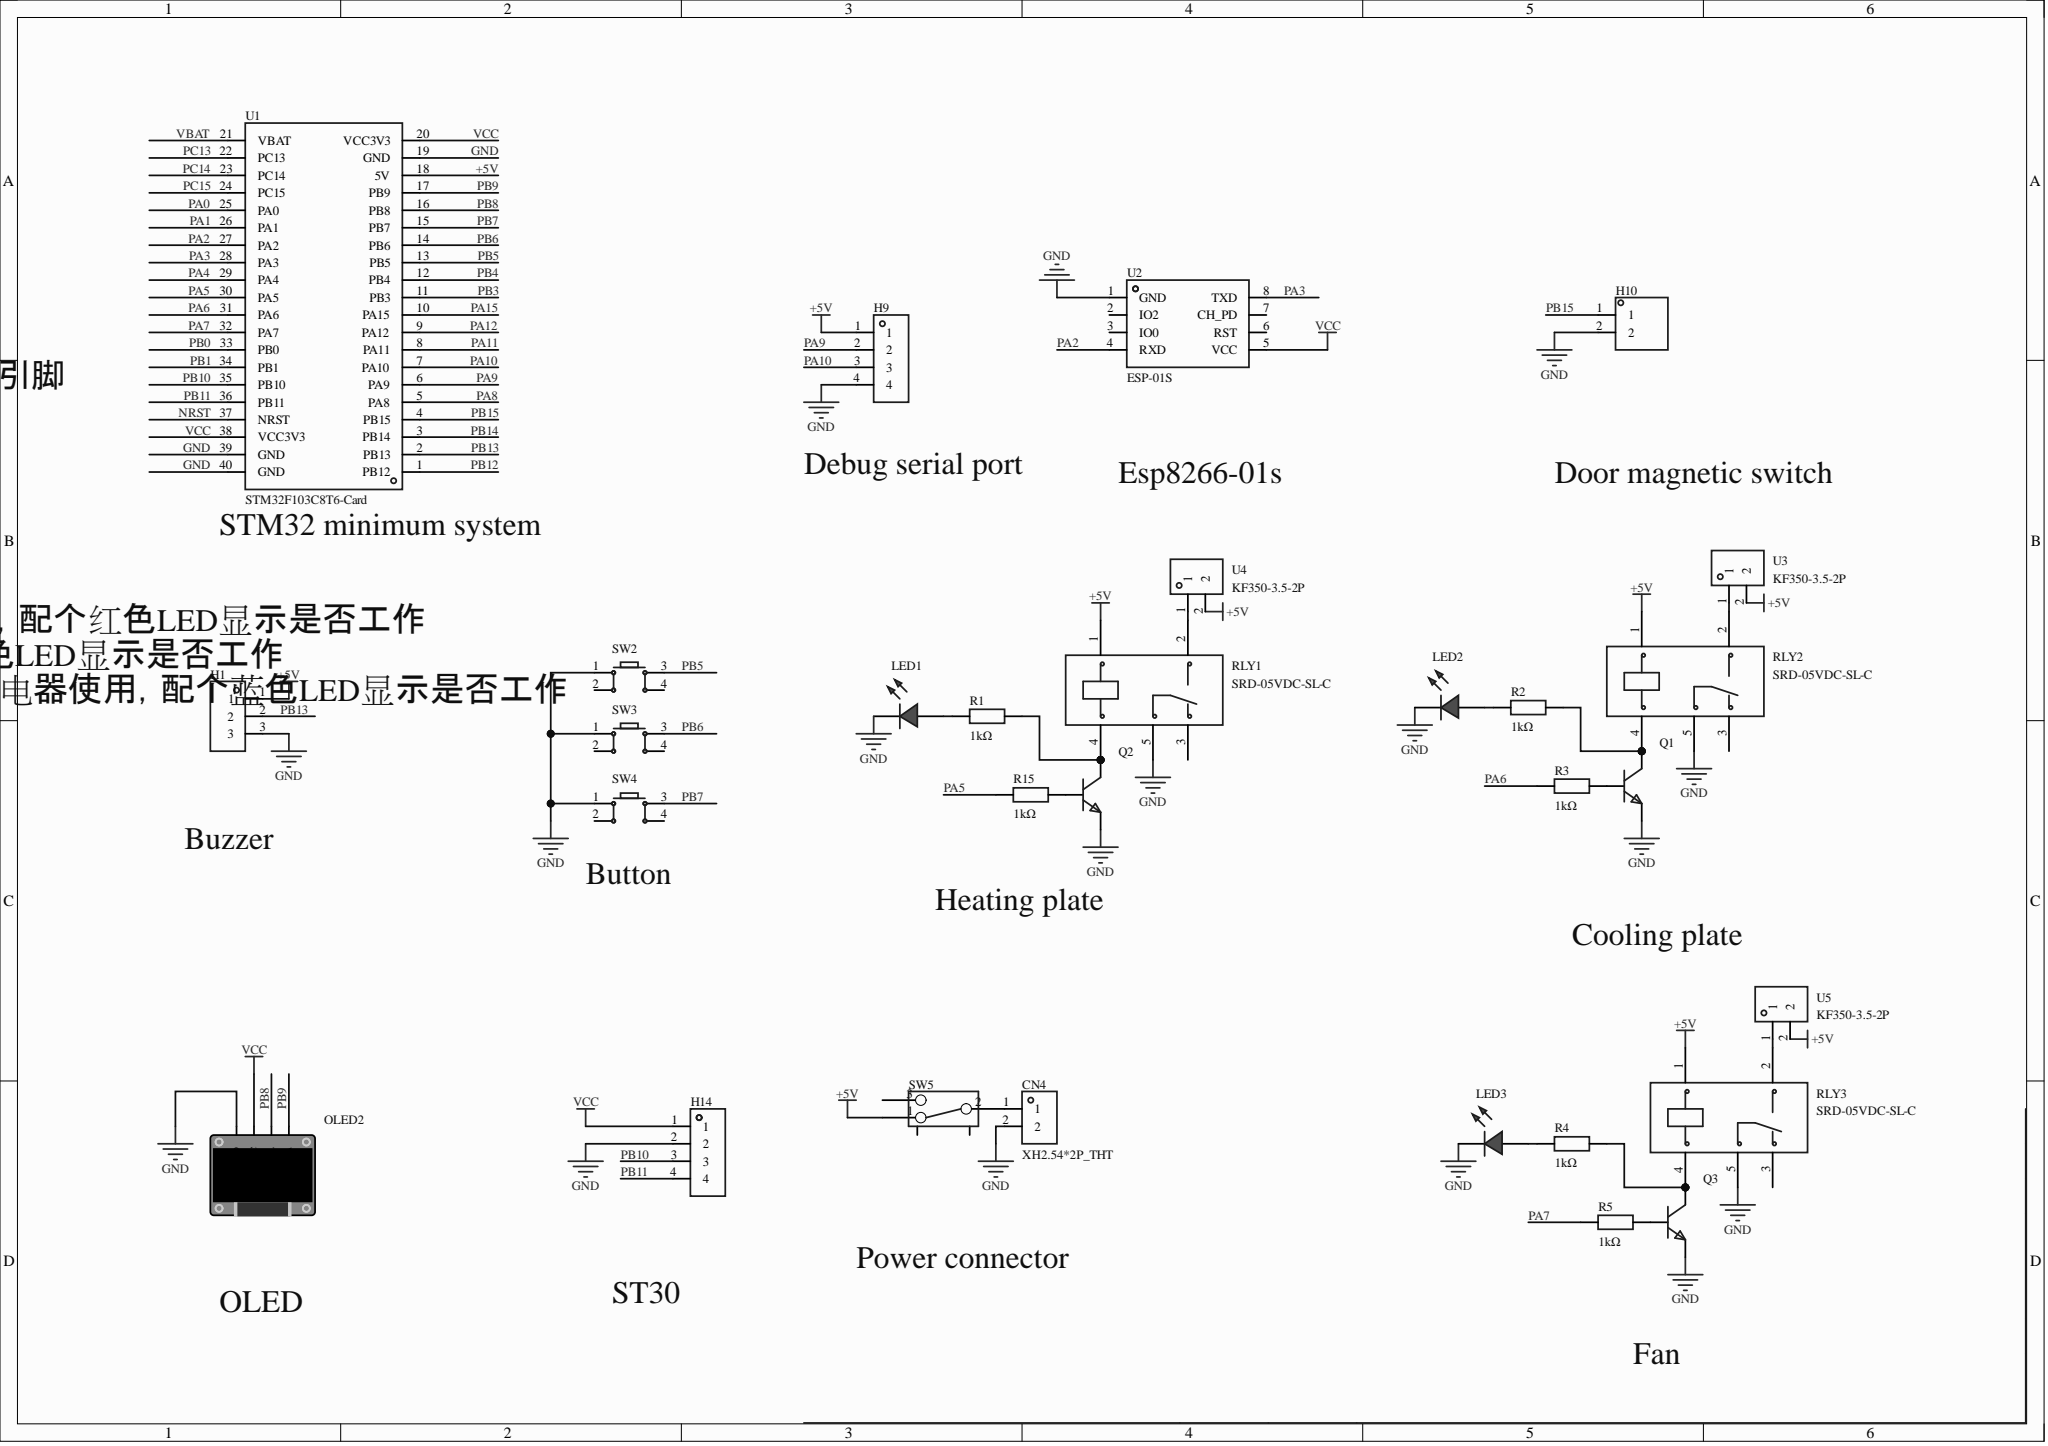Circuit board | Altium Designer | 30 parts | 32 nets
Bill of materials:
Comment,Description,Designator,Footprint,LibRef,Quantity
"XH2.54*2P_THT","","CN4","CONN-TH_2P-P2.50-XH2.54-2P","XH2.54*2P_直插","1"
"","","H1","HDR-TH_3P-P2.54-V-F","HDR-F_2.54_1x3P","1"
"","","H9","HDR-TH_4P-P2.54-V-M","HDR-M_2.54_1x4P","1"
"","","H10","HDR-TH_2P-P2.54-V-M-1","HDR-M_2.54_1x2P","1"
"","","H14","HDR-TH_4P-P2.54-V-F","HDR-F_2.54_1x4P","1"
"","","LED1, LED2, LED3","LED_TH-3mm","LED_TH-R_3mm","3"
"","","OLED2","0.96OLED_4P","0.96OLED模块_4P","1"
"","","Q1, Q2, Q3","S8050_TO_92","S8050_TO_NPN","3"
"1kΩ","","R1, R2, R3, R4, R5, R15","Res_1/4W","Res_AXIAL-1/8W","6"
"SRD-05VDC-SL-C","Coil voltage:5V;Contact form:One changeover:1C(SPDT);Contact rating(resistive load):-;Max switching voltage:250V@AC;Max switching current:15A;","RLY1, RLY2, RLY3","RELAY-TH_SRD-XXVDC-XL-C","SRD-05VDC-SL-C","3"
"","","SW2, SW3, SW4","SW-TH_4P-L6.0-W6.0-P4.50-LS6.5","Key_TH_6x6x6","3"
"","","SW5","拨动开关","拨动开关_正","1"
"STM32F103C8T6-Card","","U1","CONN-TH_L53.3-W22.9_STM32F103C8T6-CARD","STM32F103C8T6-Card","1"
"ESP-01S","","U2","WIFIM-TH_ESP-01S","ESP-01S_C111009","1"
"KF350-3.5-2P","Structure:1x2P;Pitch:3.5mm;Colour:green;Mounting:through-hole;Rated current:10A;Rated voltage:300V;Rows:1;Wire gauge - AWG:18~24;Wire gauge - mm2:0.75;Pins per row:2;Operating temperature range:-40℃~+105℃;","U3, U4, U5","CONN-TH_P3.50_KF350-3.5-2P","KF350-3.5-2P","3"
Netlist (Protel format):
[
CN4
CONN-TH_2P-P2.50-XH2.54-2P
XH2.54*2P_THT



]
[
H1
HDR-TH_3P-P2.54-V-F




]
[
H9
HDR-TH_4P-P2.54-V-M




]
[
H10
HDR-TH_2P-P2.54-V-M-1




]
[
H14
HDR-TH_4P-P2.54-V-F




]
[
LED1
LED_TH-3mm




]
[
LED2
LED_TH-3mm




]
[
LED3
LED_TH-3mm




]
[
OLED2
0.96OLED_4P




]
[
Q1
S8050_TO_92




]
[
Q2
S8050_TO_92




]
[
Q3
S8050_TO_92




]
[
R1
Res_1/4W
1kΩ



]
[
R2
Res_1/4W
1kΩ



]
[
R3
Res_1/4W
1kΩ



]
[
R4
Res_1/4W
1kΩ



]
[
R5
Res_1/4W
1kΩ



]
[
R15
Res_1/4W
1kΩ



]
[
RLY1
RELAY-TH_SRD-XXVDC-XL-C
SRD-05VDC-SL-C



]
[
RLY2
RELAY-TH_SRD-XXVDC-XL-C
SRD-05VDC-SL-C



]
[
RLY3
RELAY-TH_SRD-XXVDC-XL-C
SRD-05VDC-SL-C



]
[
SW2
SW-TH_4P-L6.0-W6.0-P4.50-LS6.5




]
[
SW3
SW-TH_4P-L6.0-W6.0-P4.50-LS6.5




]
[
SW4
SW-TH_4P-L6.0-W6.0-P4.50-LS6.5




]
[
SW5
拨动开关




]
[
U1
CONN-TH_L53.3-W22.9_STM32F103C8T6-CARD
STM32F103C8T6-Card



]
[
U2
WIFIM-TH_ESP-01S
ESP-01S



]
[
U3
CONN-TH_P3.50_KF350-3.5-2P
KF350-3.5-2P



]
[
U4
CONN-TH_P3.50_KF350-3.5-2P
KF350-3.5-2P



]
[
U5
CONN-TH_P3.50_KF350-3.5-2P
KF350-3.5-2P



]
(
VCC
H14-1
OLED2-2
U1-20
U1-38
U2-5
)
(
PB15
H10-1
U1-4
)
(
PB13
H1-2
U1-2
)
(
PB11
H14-4
U1-36
)
(
PB10
H14-3
U1-35
)
(
PB9
OLED2-4
U1-17
)
(
PB8
OLED2-3
U1-16
)
(
PB7
SW4-3
U1-15
)
(
PB6
SW3-3
U1-14
)
(
PB5
SW2-3
U1-13
)
(
PA10
H9-3
U1-7
)
(
PA9
H9-2
U1-6
)
(
PA7
R5-1
U1-32
)
(
PA6
R3-1
U1-31
)
(
PA5
R15-1
U1-30
)
(
PA3
U1-28
U2-8
)
(
PA2
U1-27
U2-4
)
(
NetRLY3_2
RLY3-2
U5-1
)
(
NetRLY2_2
RLY2-2
U3-1
)
(
NetRLY1_2
RLY1-2
U4-1
)
(
NetQ3_3
Q3-3
R4-2
RLY3-4
)
(
NetQ3_2
Q3-2
R5-2
)
(
NetQ2_3
Q2-3
R1-2
RLY1-4
)
(
NetQ2_2
Q2-2
R15-2
)
(
NetQ1_3
Q1-3
R2-2
RLY2-4
)
(
NetQ1_2
Q1-2
R3-2
)
(
NetLED3_1
LED3-1
R4-1
)
(
NetLED2_1
LED2-1
R2-1
)
(
NetLED1_1
LED1-1
R1-1
)
(
NetCN4_1
CN4-1
SW5-2
)
(
GND
CN4-2
H1-3
H9-4
H10-2
H14-2
LED1-2
LED2-2
LED3-2
OLED2-1
Q1-1
Q2-1
Q3-1
RLY1-5
RLY2-5
RLY3-5
SW2-1
SW3-1
SW4-1
U1-19
U1-39
U1-40
U2-1
)
(
+5V
H1-1
H9-1
RLY1-1
RLY2-1
RLY3-1
SW5-1
U1-18
U3-2
U4-2
U5-2
)